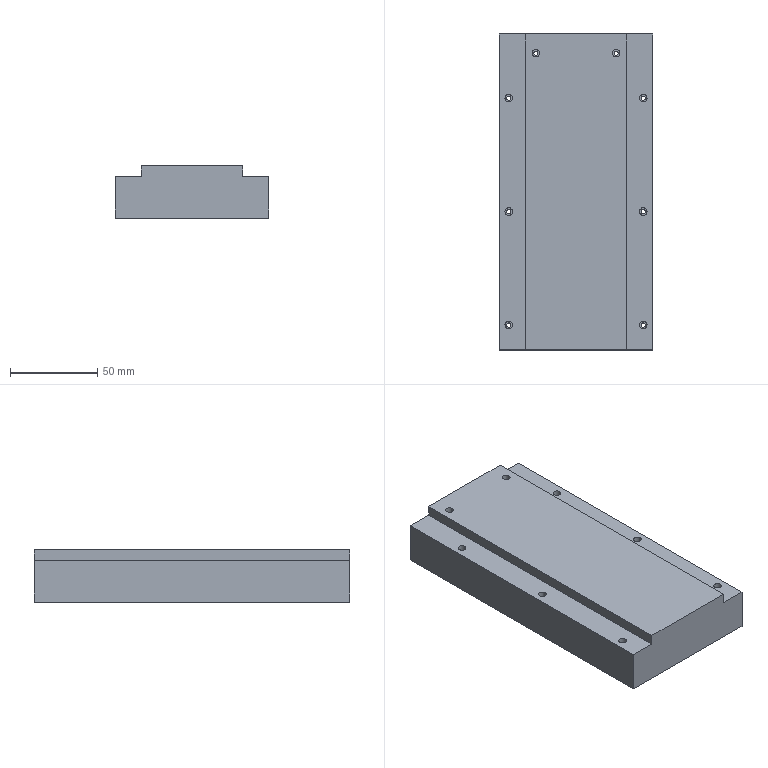NC program | NX | posted with a generic post | part box 88 x 181.05 x 30 mm
Whole program:
N10 G17 G21 G94 G90
(PLANAR_MILL , TOOL : D63_FACE_MILL)
N12 T01 M6
N14 G53
N16 G17 G0 G90 X-0.5 Y-125.025 B0. C0. S4500 M3
N18 G43 Z30. H1
N20 Z2.
N22 G94 G1 Z0. F1000.
N24 Y-90.525
N26 Y90.525
N28 Y125.025
N30 Z2.
N32 G0 Z30.
N34 M5
(DYNAMIC_ROUGH , TOOL : D16-48-D16-100-3T-ROUGH)
N36 T02 M6
N38 G53
N40 G17 G0 G90 X-57.579 Y-90.633 B0. C0. S5500 M3
N42 G43 Z30. H2
N44 Z-26.5
N46 G94 G1 X-57.554 Y-90.632 Z-26.656 F3000.
N48 X-57.529 Y-90.631 Z-26.718
N50 X-57.504 Y-90.63 Z-26.763
N52 X-57.479 Y-90.629 Z-26.8
N54 X-57.455 Y-90.627 Z-26.831
N56 X-57.43 Y-90.626 Z-26.857
N58 X-57.405 Y-90.625 Z-26.88
N60 X-57.38 Y-90.624 Z-26.9
N62 X-57.355 Y-90.623 Z-26.918
N64 X-57.33 Y-90.621 Z-26.933
N66 X-57.305 Y-90.62 Z-26.947
N68 X-57.28 Y-90.619 Z-26.958
N70 X-57.255 Y-90.618 Z-26.968
N72 X-57.23 Y-90.617 Z-26.977
N74 X-57.205 Y-90.616 Z-26.984
N76 X-57.18 Y-90.614 Z-26.99
N78 X-57.155 Y-90.613 Z-26.994
N80 X-57.13 Y-90.612 Z-26.997
N82 X-57.105 Y-90.611 Z-26.999
N84 X-57.08 Y-90.61 Z-27.
N86 X-54.472 Y-90.487
N88 G3 X-53.075 Y-89.537 R1.616
N90 X-52.43 Y-86.733 R10.15
N92 X-52.2 Y-83.934 R67.936
N94 G1 Y90.526
N96 G2 X-51.798 Y93.06 R9.591
N98 X-50.633 Y95.346 R9.588
N100 X-48.819 Y97.16 R9.588
N102 X-46.533 Y98.324 R9.588
N104 X-43.999 Y98.725 R9.593
N106 X-32.454 Y98.986 R196.191
N108 G1 X-20.754 Y98.999
N110 X41.21 Y99.
N112 G2 X43.288 Y98.73 R10.046
N114 X45.284 Y98.624 R17.692
N116 X47.724 Y97.831 R9.588
N118 X49.799 Y96.322 R9.588
N120 X51.307 Y94.247 R9.588
N122 X52.099 Y91.807 R9.588
N124 G1 X52.2 Y90.524
N126 Y-90.526
N128 G2 X51.798 Y-93.06 R9.591
N130 X50.633 Y-95.346 R9.588
N132 X48.819 Y-97.16 R9.588
N134 X46.533 Y-98.324 R9.588
N136 X43.999 Y-98.725 R9.593
N138 X32.154 Y-98.979 R208.552
N140 G1 X20.904 Y-98.992
N142 X-41.311 Y-98.998
N144 G2 X-43.313 Y-98.729 R10.858
N146 X-45.284 Y-98.624 R17.127
N148 X-47.724 Y-97.831 R9.588
N150 X-49.799 Y-96.322 R9.588
N152 X-51.307 Y-94.247 R9.588
N154 X-52.099 Y-91.807 R9.588
N156 G1 X-52.2 Y-90.524
N158 Y-83.924
N160 Y-90.524
N162 G3 X-51.799 Y-93.058 R9.591
N164 X-50.635 Y-95.344 R9.588
N166 X-48.821 Y-97.158 R9.588
N168 X-46.535 Y-98.323 R9.588
N170 X-44.001 Y-98.725 R9.59
N172 G1 X43.999
N174 G2 X45.055 Y-99.123 R1.603
N176 G1 X45.843 Y-99.815
N178 X48.221 Y-101.904 Z-26.9
N180 G3 X48.879 Y-102.348 R2.082 F15000.
N182 X50.166 Y-102.285 R1.602
N184 G1 X50.755 Y-101.993
N186 X51.337 Y-101.688
N188 G3 X52.586 Y-100.656 R5.048
N190 G1 X55.189 Y-97.678
N192 G3 X56.28 Y-95.623 R5.286
N194 X56.568 Y-94.077 R8.158
N196 G1 X56.754 Y-91.914
N198 X56.904 Y-89.749
N200 G3 X57.01 Y-86.198 R78.066
N202 G1 X58.009 Y83.924
N204 G3 X56.659 Y93.575 R33.76
N206 G1 X55.557 Y97.353
N208 G3 X54.581 Y99.002 R3.866
N210 X53.031 Y100.206 R7.93
N212 G1 X49.529 Y102.285
N214 G3 X47.677 Y102.129 R1.6
N216 G1 X45.351 Y99.983 Z-27. F3000.
N218 X44.84 Y99.506
N220 X44.317 Y99.041
N222 G2 X43.363 Y98.725 R1.605
N224 G1 X-43.999
N226 G2 X-45.511 Y99.769 R1.616
N228 G1 X-46.507 Y102.398
N230 X-46.516 Y102.422 Z-26.999
N232 X-46.525 Y102.445 Z-26.997
N234 X-46.533 Y102.468 Z-26.994
N236 X-46.542 Y102.492 Z-26.99
N238 X-46.551 Y102.515 Z-26.984
N240 X-46.56 Y102.539 Z-26.977
N242 X-46.569 Y102.562 Z-26.968
N244 X-46.578 Y102.585 Z-26.958
N246 X-46.587 Y102.609 Z-26.947
N248 X-46.595 Y102.632 Z-26.933
N250 X-46.604 Y102.655 Z-26.918
N252 X-46.613 Y102.679 Z-26.9
N254 X-46.622 Y102.702 Z-26.88
N256 X-46.631 Y102.726 Z-26.857
N258 X-46.64 Y102.749 Z-26.831
N260 X-46.649 Y102.772 Z-26.8
N262 X-46.657 Y102.796 Z-26.763
N264 X-46.666 Y102.819 Z-26.718
N266 X-46.675 Y102.842 Z-26.656
N268 X-46.684 Y102.866 Z-26.5
N270 G0 Z30.
N272 X-27.662 Y-103.175
N274 Z-5.4
N276 G1 X-27.665 Y-103.151 Z-5.556
N278 X-27.669 Y-103.126 Z-5.618
N280 X-27.672 Y-103.101 Z-5.663
N282 X-27.675 Y-103.076 Z-5.7
N284 X-27.679 Y-103.052 Z-5.731
N286 X-27.682 Y-103.027 Z-5.757
N288 X-27.686 Y-103.002 Z-5.78
N290 X-27.689 Y-102.977 Z-5.8
N292 X-27.692 Y-102.953 Z-5.818
N294 X-27.696 Y-102.928 Z-5.833
N296 X-27.699 Y-102.903 Z-5.847
N298 X-27.702 Y-102.878 Z-5.858
N300 X-27.706 Y-102.853 Z-5.868
N302 X-27.709 Y-102.829 Z-5.877
N304 X-27.713 Y-102.804 Z-5.884
N306 X-27.716 Y-102.779 Z-5.89
N308 X-27.719 Y-102.754 Z-5.894
N310 X-27.723 Y-102.73 Z-5.897
N312 X-27.726 Y-102.705 Z-5.899
N314 X-27.73 Y-102.68 Z-5.9
N316 X-28.086 Y-100.075
N318 G3 X-29.541 Y-98.685 R1.616
N320 G2 X-31.248 Y-98.389 R6.552
N322 G3 X-36.939 Y-97.859 R36.404
N324 G2 X-41.14 Y-97.737 R191.406
N326 X-46.63 Y-94.925 R8.88
N328 X-49.802 Y-89.208 R13.973
N330 X-50.922 Y-82.262 R31.9
N332 X-51.187 Y-71.017 R186.99
N334 G1 X-51.199 Y-61.042
N336 X-51.198 Y86.901
N338 G2 X-48.907 Y92.541 R8.533
N340 X-43.44 Y96.04 R13.087
N342 X-36.686 Y97.363 R27.458
N344 G1 X-33.393 Y97.572
N346 G3 X-32.896 Y97.734 R4.726
N348 X-32.094 Y98.834 R1.601
N350 G1 X-32.001 Y99.319
N352 X-31.402 Y102.427 Z-5.8
N354 X-31.332 Y102.782 F15000.
N356 X-31.277 Y103.139
N358 G3 X-32.896 Y104.854 R1.6
N360 X-33.667 Y104.739 R1.952
N362 X-33.623 Y101.747 R1.6
N364 X-32.812 Y101.666 Z-5.826 R1.799 F3000.
N366 G1 X-30.476 Y101.827 Z-5.9
N368 X-30.04 Y101.859
N370 X-29.604 Y101.876
N372 G2 X-29.541 Y98.685 R1.6
N374 G3 X-33.041 Y97.642 R7.836
N376 G2 X-35.701 Y97.035 R14.011
N378 G3 X-41.183 Y95.918 R44.607
N380 X-45.299 Y93.969 R12.692
N382 X-49.136 Y88.494 R11.803
N384 X-50.345 Y82.178 R23.998
N386 X-50.588 Y73.108 R134.382
N388 G1 X-50.599 Y64.183
N390 X-50.597 Y-64.942
N392 G3 X-50.43 Y-79.565 R388.114
N394 X-49.633 Y-86.636 R41.552
N396 X-47.833 Y-91.304 R14.579
N398 X-42.835 Y-95.395 R11.325
N400 X-37.277 Y-96.902 R22.176
N402 G2 X-33.43 Y-97.474 R557.51
N404 X-32.788 Y-97.798 R2.588
N406 G1 X-31.613 Y-98.297
N408 X-31.177 Y-98.407
N410 G2 X-33.401 Y-97.415 R7.129
N412 G3 X-36.273 Y-96.393 R15.382
N414 G2 X-40.738 Y-94.86 R28.115
N416 X-46.549 Y-89.135 R13.103
N418 X-48.77 Y-82.231 R22.213
N420 X-49.486 Y-73.341 R65.312
N422 X-49.598 Y-55.492 R785.745
N424 G1 X-49.597 Y67.108
N426 G2 X-49.452 Y79.106 R295.937
N428 X-48.643 Y85.266 R29.808
N430 X-43.491 Y92.428 R12.3
N432 X-37.725 Y95.096 R22.188
N434 G3 X-35.367 Y95.873 R98.773
N436 X-34.886 Y96.226 R2.627
N438 X-34.641 Y97.883 R1.6
N440 X-35.595 Y98.768 Z-5.858 R1.617
N442 G1 X-37.321 Y99.358 Z-5.8
N444 X-37.758 Y99.504 F15000.
N446 X-38.189 Y99.666
N448 G2 X-38.446 Y102.392 R1.6
N450 G1 X-38.155 Y102.61
N452 X-37.856 Y102.816
N454 G2 X-36.107 Y102.716 R1.6
N456 G1 X-34.381 Y101.44
N458 X-32.801 Y100.265 Z-5.862 F3000.
N460 G2 X-32.237 Y99.244 Z-5.9 R1.6
N462 X-32.976 Y97.68 R1.6
N464 G3 X-35.029 Y96.06 R7.847
N466 G2 X-36.762 Y95.084 R7.614
N468 G3 X-41.137 Y92.939 R42.882
N470 X-47.329 Y85.319 R14.067
N472 X-48.679 Y78.496 R26.941
N474 X-48.983 Y68.753 R129.201
N476 G1 X-48.998 Y59.078
N478 X-48.996 Y-59.172
N480 G3 X-48.83 Y-74.32 R437.01
N482 X-48.002 Y-82.37 R51.912
N484 X-45.631 Y-88.734 R19.104
N486 X-40.141 Y-93.77 R14.478
N488 X-35.55 Y-95.849 R48.344
N490 G2 X-34.858 Y-96.259 R2.394
N492 X-34.522 Y-97.637 R1.601
N494 X-34.98 Y-98.456 Z-5.87 R1.755
N496 G1 X-36.432 Y-100.128 Z-5.8
N498 X-38.327 Y-102.309 F15000.
N500 G3 X-36.849 Y-104.957 R1.604
N502 X-35.78 Y-104.232 R1.602
N504 G1 X-34.105 Y-101.558
N506 X-32.85 Y-99.544 Z-5.875 F3000.
N508 G3 X-32.648 Y-98.788 Z-5.9 R1.606
N510 X-33.401 Y-97.415 R1.601
N512 G2 X-35.029 Y-96.057 R7.102
N514 G3 X-37.102 Y-94.559 R13.304
N516 G2 X-41.245 Y-91.517 R25.827
N518 X-46.005 Y-83.797 R18.407
N520 X-47.566 Y-75.486 R36.355
N522 X-47.964 Y-64.396 R149.197
N524 G1 X-47.997 Y-49.846
N526 X-47.996 Y62.029
N528 G2 X-47.833 Y74.927 R309.518
N530 X-46.958 Y81.836 R36.18
N532 X-41.207 Y90.707 R15.688
N534 X-37.224 Y93.434 R49.413
N536 G3 X-36.32 Y94.219 R2.677
N538 X-36.485 Y95.731 R1.601
N540 X-37.618 Y96.419 Z-5.857 R1.679
N542 G1 X-39.379 Y96.791 Z-5.8
N544 X-39.912 Y96.9 F15000.
N546 X-40.441 Y97.027
N548 G2 X-41.355 Y99.254 R1.6
N550 G1 X-41.208 Y99.553
N552 X-41.048 Y99.845
N554 G2 X-38.979 Y100.384 R1.6
N556 G1 X-37.225 Y99.478
N558 X-35.394 Y98.527 Z-5.865 F3000.
N560 G2 X-34.7 Y97.701 Z-5.9 R1.601
N562 X-34.979 Y96.116 R1.601
N564 G1 X-35.657 Y95.312
N566 X-36.427 Y94.024
N568 G2 X-38.244 Y92.338 R11.446
N570 G3 X-42.213 Y88.719 R30.381
N572 X-46.224 Y80.707 R18.633
N574 X-47.202 Y73.131 R40.97
N576 X-47.393 Y61.059 R266.297
N578 G1 X-47.397 Y55.509
N580 X-47.395 Y-54.491
N582 G3 X-47.224 Y-70.539 R479.067
N584 X-46.319 Y-79.56 R59.081
N586 X-43.601 Y-86.988 R22.788
N588 X-38.701 Y-92.39 R20.469
N590 G2 X-36.307 Y-94.305 R71.67
N592 X-35.659 Y-95.311 R6.411
N594 G1 X-34.981 Y-96.113
N596 G2 X-36.154 Y-94.495 R7.587
N598 G3 X-38. Y-92.16 R13.26
N600 G2 X-41.934 Y-87.122 R30.771
N602 X-45.226 Y-78.145 R27.23
N604 X-46.199 Y-68.528 R64.957
N606 X-46.392 Y-53.68 R418.722
N608 G1 X-46.396 Y-47.23
N610 X-46.395 Y58.12
N612 G2 X-46.224 Y71.543 R328.441
N614 X-45.287 Y79.2 R41.789
N616 X-40.223 Y88.601 R20.398
N618 G3 X-37.288 Y91.723 R211.462
N620 X-36.977 Y92.317 R2.167
N622 G1 X-36.805 Y93.04
N624 X-36.32 Y94.221
N626 X-36.805 Y93.04
N628 G2 X-37.133 Y91.859 R5.847
N630 X-38.688 Y89.653 R14.553
N632 G3 X-42.088 Y84.891 R35.69
N634 X-45.011 Y76.194 R25.459
N636 X-45.709 Y67.003 R68.975
N638 X-45.796 Y52.153 R780.496
N640 G1 X-45.794 Y-50.872
N642 G3 X-45.618 Y-67.445 R507.889
N644 X-44.68 Y-77.216 R67.586
N646 X-41.201 Y-86.677 R27.532
N648 X-37.798 Y-91.331 R44.339
N650 G2 X-36.937 Y-92.557 R6.424
N652 G3 X-36.321 Y-94.219 R10.442
N654 G1 X-36.805 Y-93.038
N656 G3 X-37.803 Y-90.538 R7.763
N658 G2 X-40.562 Y-85.586 R97.842
N660 X-43.9 Y-74.327 R36.607
N662 X-44.68 Y-63.11 R97.377
N664 X-44.795 Y-42.861 R960.397
N666 G1 X-44.794 Y54.689
N668 G2 X-44.614 Y68.712 R346.85
N670 X-43.615 Y77.116 R47.758
N672 X-39.681 Y86.157 R27.035
N674 G3 X-37.365 Y89.78 R62.753
N676 X-37.2 Y90.526 R1.886
N678 G1 X-37.1 Y91.799
N680 X-36.996 Y92.236
N682 X-37.1 Y91.799
N684 G3 X-37.202 Y90.205 R30.629
N686 G2 X-38.003 Y88.147 R7.219
N688 G3 X-40.578 Y83.342 R148.541
N690 X-43.578 Y72.699 R33.082
N692 X-44.137 Y62.67 R96.58
N694 X-44.195 Y49.02 R824.817
N696 G1 X-44.193 Y-47.555
N698 G3 X-43.996 Y-65.253 R514.765
N700 X-42.956 Y-75.842 R73.395
N702 X-38.768 Y-87.44 R38.406
N704 G2 X-37.249 Y-90.463 R40.428
N706 X-37.101 Y-91.796 R7.37
N708 G1 X-36.962 Y-92.38
N710 G2 X-37.182 Y-90.755 R6.826
N712 G3 X-37.785 Y-88.183 R8.487
N714 G2 X-40. Y-82.353 R344.373
N716 X-42.626 Y-69.522 R52.699
N718 X-43.15 Y-56.035 R172.474
N720 G1 X-43.193 Y-42.985
N722 X-43.194 Y49.015
N724 G2 X-43.042 Y65.363 R503.011
N726 X-42.06 Y74.902 R59.741
N728 X-38.84 Y84.089 R37.509
N730 G3 X-37.263 Y87.577 R44.436
N732 G1 X-37.2 Y87.946
N734 Y90.346
N736 Y87.721
N738 G2 X-38.01 Y84.934 R11.897
N740 G3 X-40.253 Y78.95 R94.427
N742 X-42.228 Y67.976 R47.273
N744 X-42.58 Y55.233 R191.566
N746 G1 X-42.594 Y45.633
N748 X-42.592 Y-44.492
N750 G3 X-42.393 Y-62.94 R557.266
N752 X-41.306 Y-74.504 R84.598
N754 X-38.407 Y-84.74 R56.515
N756 G2 X-37.213 Y-88.338 R32.946
N758 G1 X-37.2 Y-90.513
N760 G3 X-37.227 Y-87.289 R48.809
N762 X-38.108 Y-83.238 R27.601
N764 G2 X-40.368 Y-73.316 R85.738
N766 X-41.424 Y-60.392 R104.045
N768 X-41.591 Y-42.244 R677.387
N770 G1 X-41.593 Y46.006
N772 G2 X-41.442 Y62.955 R552.269
N774 X-40.382 Y73.616 R68.567
N776 X-38.079 Y81.685 R54.328
N778 G3 X-37.217 Y84.299 R32.425
N780 X-37.2 Y87.748 R75.884
N782 G1 X-37.216 Y83.983
N784 G2 X-38.078 Y80.196 R25.33
N786 G3 X-40.743 Y64.073 R65.145
N788 X-40.988 Y49.527 R317.354
N790 G1 X-40.992 Y43.302
N792 X-40.991 Y-41.723
N794 G3 X-40.785 Y-61.071 R595.252
N796 X-39.534 Y-74.276 R96.031
N798 X-37.638 Y-82.619 R110.394
N800 G2 X-37.2 Y-84.591 R26.785
N802 G1 Y-87.666
N804 G3 X-37.221 Y-82.574 R148.285
N806 X-37.777 Y-78.578 R47.276
N808 G2 X-39.819 Y-58.523 R122.634
N810 X-39.99 Y-38.574 R784.404
N812 G1 X-39.992 Y43.751
N814 G2 X-39.821 Y61.299 R541.407
N816 X-38.553 Y73.521 R77.38
N818 X-37.213 Y79.398 R165.87
N820 G1 X-37.2 Y84.273
N822 X-37.213 Y78.685
N824 G2 X-37.956 Y73.588 R61.471
N826 G3 X-39.272 Y58.509 R103.852
N828 X-39.391 Y40.96 R809.745
N830 G1 Y-74.951
N832 G2 X-39.518 Y-75.575 R1.631
N834 G1 X-39.922 Y-76.529
N836 X-41.155 Y-79.444 Z-5.8
N838 X-41.338 Y-79.881 F15000.
N840 X-41.535 Y-80.311
N842 G2 X-42.951 Y-81.117 R1.601
N844 G1 X-44.078 Y-81.098
N846 G3 X-44.179 Y-84.296 R1.6
N848 G1 X-41.175 Y-84.434
N850 X-38.787 Y-84.539 Z-5.876 F3000.
N852 G3 X-38.044 Y-84.351 Z-5.9 R1.607
N854 X-37.2 Y-82.941 R1.601
N856 X-37.229 Y-78.107 R108.816
N858 X-38.004 Y-70.447 R255.912
N860 G2 X-38.337 Y-60.331 R110.883
N862 G1 X-38.341 Y-53.731
N864 X-38.34 Y70.926
N866 G3 X-38.436 Y71.471 R1.672
N868 G1 X-39.64 Y74.79
N870 X-39.97 Y75.705 Z-5.869
N872 X-40.309 Y76.617 Z-5.838
N874 G3 X-41.149 Y77.458 Z-5.8 R1.6
N876 X-43.375 Y75.961 R1.6 F15000.
N878 G1 X-43.372 Y75.577
N880 X-43.352 Y75.195
N882 G3 X-41.171 Y73.928 R1.6
N884 X-40.17 Y75.521 Z-5.864 R1.606 F3000.
N886 G1 X-40.249 Y76.671 Z-5.9
N888 X-40.396 Y78.839
N890 G2 X-37.2 Y78.948 R-1.6
N892 X-37.476 Y73.301 R40.731
N894 G3 X-37.727 Y64.157 R129.856
N896 G1 X-37.74 Y54.407
N898 X-37.736 Y-70.751
N900 G2 X-37.2 Y-73.643 R55.721
N902 G1 Y-78.668
N904 Y76.807
N906 G3 X-38.586 Y78.407 R1.616
N908 G1 X-41.156 Y78.777
N910 X-41.181 Y78.781 Z-5.899
N912 X-41.205 Y78.784 Z-5.897
N914 X-41.23 Y78.788 Z-5.894
N916 X-41.255 Y78.791 Z-5.89
N918 X-41.279 Y78.795 Z-5.884
N920 X-41.304 Y78.798 Z-5.877
N922 X-41.329 Y78.802 Z-5.868
N924 X-41.354 Y78.806 Z-5.858
N926 X-41.378 Y78.809 Z-5.847
N928 X-41.403 Y78.813 Z-5.833
N930 X-41.428 Y78.816 Z-5.818
N932 X-41.453 Y78.82 Z-5.8
N934 X-41.477 Y78.823 Z-5.78
N936 X-41.502 Y78.827 Z-5.757
N938 X-41.527 Y78.831 Z-5.731
N940 X-41.552 Y78.834 Z-5.7
N942 X-41.576 Y78.838 Z-5.663
N944 X-41.601 Y78.841 Z-5.618
N946 X-41.626 Y78.845 Z-5.556
N948 X-41.651 Y78.848 Z-5.4
N950 G0 Z30.
N952 X27.662 Y103.175
N954 Z-5.4
N956 G1 X27.665 Y103.151 Z-5.556
N958 X27.669 Y103.126 Z-5.618
N960 X27.672 Y103.101 Z-5.663
N962 X27.675 Y103.076 Z-5.7
N964 X27.679 Y103.052 Z-5.731
N966 X27.682 Y103.027 Z-5.757
N968 X27.686 Y103.002 Z-5.78
N970 X27.689 Y102.977 Z-5.8
N972 X27.692 Y102.953 Z-5.818
N974 X27.696 Y102.928 Z-5.833
N976 X27.699 Y102.903 Z-5.847
N978 X27.702 Y102.878 Z-5.858
N980 X27.706 Y102.853 Z-5.868
N982 X27.709 Y102.829 Z-5.877
N984 X27.713 Y102.804 Z-5.884
N986 X27.716 Y102.779 Z-5.89
N988 X27.719 Y102.754 Z-5.894
N990 X27.723 Y102.73 Z-5.897
N992 X27.726 Y102.705 Z-5.899
N994 X27.73 Y102.68 Z-5.9
N996 X28.086 Y100.075
N998 G3 X29.541 Y98.685 R1.616
N1000 G2 X31.248 Y98.389 R6.552
N1002 G3 X36.543 Y97.876 R34.52
N1004 G2 X41.088 Y97.742 R627.78
N1006 X46.582 Y94.936 R8.89
N1008 X49.741 Y89.336 R13.941
N1010 X50.901 Y82.473 R30.771
N1012 X51.183 Y71.828 R166.117
N1014 G1 X51.199 Y61.028
N1016 Y-86.851
N1018 G2 X48.762 Y-92.735 R8.576
N1020 X43.264 Y-96.124 R13.244
N1022 X36.572 Y-97.379 R28.234
N1024 G1 X33.355 Y-97.582
N1026 G3 X32.86 Y-97.752 R4.815
N1028 X32.155 Y-98.736 R1.602
N1030 G1 X32.002 Y-99.379
N1032 X31.268 Y-102.457 Z-5.8
N1034 X31.191 Y-102.774 F15000.
N1036 X31.127 Y-103.094
N1038 G3 X32.86 Y-104.873 R1.6
N1040 X33.479 Y-104.77 R2.34
N1042 X33.563 Y-101.776 R1.6
N1044 X32.695 Y-101.672 Z-5.828 R1.773 F3000.
N1046 G1 X30.42 Y-101.831 Z-5.9
N1048 X30.013 Y-101.862
N1050 X29.605 Y-101.876
N1052 G2 X29.541 Y-98.685 R1.6
N1054 G3 X33.041 Y-97.642 R7.841
N1056 G2 X35.714 Y-97.039 R14.327
N1058 G3 X41.196 Y-95.932 R45.055
N1060 X45.428 Y-93.896 R12.469
N1062 X49.132 Y-88.537 R11.814
N1064 X50.344 Y-82.222 R23.955
N1066 X50.587 Y-73.228 R132.894
N1068 G1 X50.599 Y-64.453
N1070 X50.597 Y64.897
N1072 G3 X50.447 Y79.071 R418.723
N1074 X49.675 Y86.371 R44.128
N1076 X47.797 Y91.325 R15.044
N1078 X42.739 Y95.43 R11.289
N1080 X37.176 Y96.918 R22.397
N1082 G2 X33.419 Y97.477 R241.725
N1084 X32.788 Y97.798 R2.67
N1086 G1 X31.613 Y98.297
N1088 X31.177 Y98.407
N1090 G2 X33.391 Y97.421 R7.119
N1092 G3 X36.355 Y96.369 R15.586
N1094 G2 X40.792 Y94.826 R26.912
N1096 X46.558 Y89.092 R13.158
N1098 X48.772 Y82.191 R22.279
N1100 X49.48 Y73.527 R64.425
N1102 X49.598 Y57.403 R667.953
N1104 G1 Y-64.747
N1106 G2 X49.475 Y-78.621 R416.586
N1108 X48.752 Y-84.87 R33.205
N1110 X43.453 Y-92.472 R12.305
N1112 X37.733 Y-95.102 R22.213
N1114 G3 X35.371 Y-95.875 R182.58
N1116 X34.887 Y-96.224 R2.691
N1118 X34.641 Y-97.883 R1.6
N1120 X35.595 Y-98.768 Z-5.858 R1.617
N1122 G1 X37.322 Y-99.357 Z-5.8
N1124 X37.758 Y-99.504 F15000.
N1126 X38.188 Y-99.665
N1128 G2 X38.447 Y-102.391 R1.6
N1130 G1 X38.156 Y-102.609
N1132 X37.856 Y-102.816
N1134 G2 X36.106 Y-102.716 R1.6
N1136 G1 X34.381 Y-101.44
N1138 X32.801 Y-100.265 Z-5.862 F3000.
N1140 G2 X32.237 Y-99.243 Z-5.9 R1.6
N1142 X32.976 Y-97.68 R1.6
N1144 G3 X35.029 Y-96.06 R7.891
N1146 G2 X36.95 Y-95.004 R8.663
N1148 G3 X41.323 Y-92.84 R37.076
N1150 X47.332 Y-85.335 R14.038
N1152 X48.693 Y-78.362 R27.229
N1154 X48.983 Y-68.844 R131.936
N1156 G1 X48.998 Y-59.169
N1158 X48.996 Y58.856
N1160 G3 X48.829 Y74.304 R444.778
N1162 X47.969 Y82.5 R51.129
N1164 X45.548 Y88.847 R18.885
N1166 X39.975 Y93.855 R14.629
N1168 X35.508 Y95.866 R51.692
N1170 G2 X34.879 Y96.238 R2.518
N1172 X34.497 Y97.714 R1.601
N1174 X35.196 Y98.69 Z-5.861 R1.695
N1176 G1 X36.734 Y99.867 Z-5.8
N1178 X37.863 Y100.73 F15000.
N1180 G3 X38.426 Y102.456 R1.603
N1182 X35.632 Y103.057 R1.6
N1184 G1 X34.341 Y101.456
N1186 X32.943 Y99.714 Z-5.871 F3000.
N1188 G3 X32.64 Y98.849 Z-5.9 R1.603
N1190 X33.391 Y97.421 R1.601
N1192 G2 X35.029 Y96.057 R7.112
N1194 G3 X37.057 Y94.584 R12.939
N1196 G2 X41.164 Y91.585 R26.33
N1198 X45.966 Y83.895 R18.379
N1200 X47.548 Y75.664 R35.768
N1202 X47.963 Y64.424 R145.593
N1204 G1 X47.997 Y49.875
N1206 X47.996 Y-62.075
N1208 G2 X47.828 Y-75.048 R303.462
N1210 X46.915 Y-82.027 R35.159
N1212 X41.153 Y-90.763 R15.679
N1214 X37.165 Y-93.482 R52.04
N1216 G3 X36.304 Y-94.247 R2.491
N1218 G2 X34.931 Y-96.172 R9.009
N1220 G3 X36.304 Y-94.247 R9.039
N1222 G2 X37.117 Y-93.3 R3.297
N1224 G1 X40.343 Y-90.602
N1226 G3 X46.163 Y-80.972 R18.329
N1228 X47.205 Y-73.103 R40.233
N1230 X47.393 Y-61.106 R268.747
N1232 G1 X47.397 Y-55.556
N1234 X47.395 Y54.519
N1236 G3 X47.221 Y70.567 R473.769
N1238 X46.31 Y79.587 R58.808
N1240 X43.532 Y87.087 R22.654
N1242 X38.699 Y92.387 R20.534
N1244 G2 X36.336 Y94.272 R349.742
N1246 X35.659 Y95.311 R7.101
N1248 G1 X34.981 Y96.113
N1250 G2 X36.148 Y94.504 R7.558
N1252 G3 X37.989 Y92.168 R13.256
N1254 G2 X42.002 Y86.996 R30.481
N1256 X45.223 Y78.14 R27.313
N1258 X46.199 Y68.523 R64.871
N1260 X46.391 Y53.75 R414.218
N1262 G1 X46.396 Y47.225
N1264 X46.395 Y-58.2
N1266 G2 X46.213 Y-71.773 R314.86
N1268 X45.22 Y-79.496 R40.261
N1270 X40.26 Y-88.57 R20.315
N1272 G3 X37.264 Y-91.758 R206.313
N1274 X36.978 Y-92.312 R2.424
N1276 G1 X36.805 Y-93.04
N1278 X36.32 Y-94.221
N1280 X36.805 Y-93.04
N1282 G2 X37.133 Y-91.863 R5.732
N1284 X38.693 Y-89.654 R14.741
N1286 G3 X42.116 Y-84.857 R35.229
N1288 X45.021 Y-76.153 R25.489
N1290 X45.712 Y-66.886 R69.977
N1292 X45.796 Y-52.111 R799.078
N1294 G1 X45.794 Y50.839
N1296 G3 X45.618 Y67.412 R508.303
N1298 X44.723 Y76.962 R68.853
N1300 X41.451 Y86.251 R27.994
N1302 X37.889 Y91.212 R40.398
N1304 G2 X36.962 Y92.497 R8.541
N1306 G3 X36.321 Y94.219 R12.516
N1308 G1 X36.805 Y93.038
N1310 G3 X37.862 Y90.43 R8.113
N1312 G2 X40.68 Y85.336 R83.784
N1314 X43.907 Y74.272 R36.784
N1316 X44.681 Y63.055 R97.954
N1318 X44.795 Y42.731 R965.467
N1320 G1 X44.794 Y-54.669
N1322 G2 X44.619 Y-68.617 R354.967
N1324 X43.672 Y-76.878 R48.986
N1326 X39.697 Y-86.142 R26.952
N1328 G3 X37.373 Y-89.77 R65.981
N1330 X37.2 Y-90.526 R1.874
N1332 G1 X37.1 Y-91.799
N1334 X36.996 Y-92.237
N1336 X37.1 Y-91.799
N1338 G3 X37.202 Y-90.193 R32.486
N1340 G2 X38.015 Y-88.131 R7.559
N1342 G3 X40.597 Y-83.314 R138.376
N1344 X43.566 Y-72.815 R32.949
N1346 X44.136 Y-62.711 R95.406
N1348 X44.195 Y-48.386 R847.301
N1350 G1 X44.193 Y47.364
N1352 G3 X44.009 Y64.912 R539.736
N1354 X43.002 Y75.581 R75.896
N1356 X38.747 Y87.472 R38.588
N1358 G2 X37.233 Y90.513 R30.005
N1360 X37.101 Y91.796 R9.107
N1362 G1 X36.962 Y92.38
N1364 G2 X37.183 Y90.743 R6.891
N1366 G3 X37.776 Y88.201 R8.423
N1368 G2 X39.892 Y82.653 R627.127
N1370 X42.602 Y69.769 R52.175
N1372 X43.144 Y56.659 R163.853
N1374 X43.193 Y42.934 R886.056
N1376 G1 X43.194 Y-48.691
N1378 G2 X43.049 Y-65.19 R533.095
N1380 X42.112 Y-74.658 R61.228
N1382 X38.989 Y-83.786 R36.599
N1384 G3 X37.26 Y-87.594 R45.39
N1386 G1 X37.2 Y-87.963
N1388 Y-90.288
N1390 Y-87.738
N1392 G2 X38.021 Y-84.915 R11.769
N1394 G3 X40.334 Y-78.709 R88.089
N1396 X42.237 Y-67.872 R47.671
N1398 X42.579 Y-55.279 R194.072
N1400 G1 X42.594 Y-45.679
N1402 X42.592 Y44.446
N1404 G3 X42.397 Y62.819 R564.791
N1406 X41.299 Y74.533 R84.986
N1408 X38.625 Y84.134 R54.44
N1410 G2 X37.218 Y88.301 R43.745
N1412 X37.2 Y90.478 R53.698
N1414 G1 X37.214 Y87.417
N1416 G3 X38.012 Y83.588 R23.777
N1418 G2 X40.128 Y74.743 R97.896
N1420 X41.375 Y61.838 R93.104
N1422 X41.589 Y43.915 R528.791
N1424 G1 X41.593 Y37.315
N1426 X41.592 Y-48.385
N1428 G2 X41.397 Y-64.132 R403.887
N1430 X40.162 Y-74.697 R61.584
N1432 X37.878 Y-82.264 R61.028
N1434 G3 X37.209 Y-84.363 R16.695
N1436 G1 X37.2 Y-87.764
N1438 G2 X37.22 Y-83.923 R100.459
N1440 X38.026 Y-80.394 R25.08
N1442 G3 X40.291 Y-69.659 R65.632
N1444 X40.922 Y-58.506 R112.739
N1446 X40.993 Y-43.207 R858.341
N1448 G1 X40.991 Y41.743
N1450 G3 X40.786 Y61.016 R595.386
N1452 X39.555 Y74.149 R96.628
N1454 X37.635 Y82.62 R109.055
N1456 G2 X37.2 Y84.584 R23.554
N1458 G1 Y87.659
N1460 G3 X37.224 Y82.531 R132.32
N1462 X38.087 Y76.772 R68.277
N1464 G2 X39.813 Y58.721 R120.013
N1466 X39.99 Y39.223 R742.571
N1468 G1 X39.992 Y-43.702
N1470 G2 X39.818 Y-61.4 R542.426
N1472 X38.478 Y-73.914 R76.332
N1474 X37.207 Y-79.456 R268.848
N1476 G1 X37.2 Y-84.181
N1478 X37.21 Y-78.757
N1480 G2 X37.852 Y-74.229 R50.064
N1482 G3 X39.271 Y-58.558 R103.393
N1484 X39.391 Y-39.659 R867.629
N1486 G1 Y73.301
N1488 G2 X39.481 Y73.828 R1.684
N1490 G1 X40.096 Y75.592
N1492 X41.087 Y78.434 Z-5.805
N1494 X41.145 Y78.578 Z-5.8
N1496 G2 X42.952 Y79.467 R1.6 F15000.
N1498 G1 X43.252 Y79.399
N1500 X43.554 Y79.342
N1502 G3 X44.323 Y82.416 R1.6
N1504 G1 X41.175 Y83.695
N1506 X39.318 Y84.445 Z-5.863 F3000.
N1508 G3 X38.183 Y84.41 Z-5.9 R1.6
N1510 X37.2 Y82.934 R1.6
N1512 X37.226 Y78.182 R122.277
N1514 X37.972 Y70.77 R205.442
N1516 G2 X38.337 Y60.355 R105.883
N1518 G1 X38.341 Y53.455
N1520 Y-70.976
N1522 G3 X38.436 Y-71.521 R1.672
N1524 G1 X39.64 Y-74.841
N1526 X39.97 Y-75.756 Z-5.869
N1528 X40.309 Y-76.668 Z-5.838
N1530 G3 X41.149 Y-77.509 Z-5.8 R1.6
N1532 X43.376 Y-76.011 R1.6 F15000.
N1534 G1 X43.372 Y-75.631
N1536 X43.352 Y-75.253
N1538 G3 X41.171 Y-73.986 R1.6
N1540 X40.17 Y-75.58 Z-5.864 R1.606 F3000.
N1542 G1 X40.249 Y-76.73 Z-5.9
N1544 X40.396 Y-78.897
N1546 G2 X37.2 Y-79.006 R-1.6
N1548 X37.454 Y-73.573 R36.404
N1550 G3 X37.722 Y-65.18 R111.834
N1552 G1 X37.74 Y-54.38
N1554 X37.736 Y69.176
N1556 G2 X37.2 Y72.876 R223.56
N1558 G1 Y78.801
N1560 Y-76.824
N1562 G3 X38.586 Y-78.424 R1.616
N1564 G1 X41.156 Y-78.794
N1566 X41.181 Y-78.797 Z-5.899
N1568 X41.205 Y-78.801 Z-5.897
N1570 X41.23 Y-78.804 Z-5.894
N1572 X41.255 Y-78.808 Z-5.89
N1574 X41.279 Y-78.812 Z-5.884
N1576 X41.304 Y-78.815 Z-5.877
N1578 X41.329 Y-78.819 Z-5.868
N1580 X41.354 Y-78.822 Z-5.858
N1582 X41.378 Y-78.826 Z-5.847
N1584 X41.403 Y-78.829 Z-5.833
N1586 X41.428 Y-78.833 Z-5.818
N1588 X41.453 Y-78.836 Z-5.8
N1590 X41.477 Y-78.84 Z-5.78
N1592 X41.502 Y-78.844 Z-5.757
N1594 X41.527 Y-78.847 Z-5.731
N1596 X41.552 Y-78.851 Z-5.7
N1598 X41.576 Y-78.854 Z-5.663
N1600 X41.601 Y-78.858 Z-5.618
N1602 X41.626 Y-78.861 Z-5.556
N1604 X41.651 Y-78.865 Z-5.4
N1606 G0 Z30.
N1608 M5
(PLANAR_MILL_1 , TOOL : D16-48-D16-100-3T-FINISH)
N1610 T03 M6
N1612 G53
N1614 G17 G0 G90 X-43.4 Y-106.525 B0. C0. S4500 M3
N1616 G43 Z30. H3
N1618 Z-3.
N1620 G94 G1 Z-6. F1000.
N1622 Y-90.525
N1624 Y90.525
N1626 Y106.525
N1628 Z-3.
N1630 G0 Z30.
N1632 X-37. Y-106.525
N1634 Z-3.
N1636 G1 Z-6.
N1638 Y-90.525
N1640 Y90.525
N1642 Y106.525
N1644 Z-3.
N1646 G0 Z30.
N1648 X43.4
N1650 Z-3.
N1652 G1 Z-6.
N1654 Y90.525
N1656 Y-90.525
N1658 Y-106.525
N1660 Z-3.
N1662 G0 Z30.
N1664 X37. Y106.525
N1666 Z-3.
N1668 G1 Z-6.
N1670 Y90.525
N1672 Y-90.525
N1674 Y-106.525
N1676 Z-3.
N1678 G0 Z30.
(PLANAR_MILL_1_COPY , TOOL : D16-48-D16-100-3T-FINISH)
N1680 X-57.856 Y98.525
N1682 Z-24.
N1684 G1 Z-27.
N1686 X-43.997
N1688 X44.
N1690 G2 X52. Y90.525 R8.
N1692 G1 Y-90.525
N1694 G2 X44. Y-98.525 R8.
N1696 G1 X-44.
N1698 G2 X-52. Y-90.525 R8.
N1700 G1 Y90.522
N1702 Y104.381
N1704 Z-24.
N1706 G0 Z30.
N1708 M5
(DRILLING , TOOL : CHAMFER_D6-90DEG)
N1710 T04 M6
N1712 G53
N1714 G17 G0 G90 X23. Y79.525 B0. C0. S3000 M3
N1716 G43 Z30. H4
N1718 G94 G81 G99 Z-2.2 F200. R3.
N1720 X-23.
N1722 G80
N1724 G0 X-23. Y79.525 Z30.
(DRILLING_COPY , TOOL : CHAMFER_D6-90DEG)
N1726 X38.5 Y53.775
N1728 G81 G98 Z-8.2 F200. R-3.
N1730 Y-11.225
N1732 Y-76.225
N1734 X-38.5
N1736 Y-11.225
N1738 Y53.775
N1740 G80
N1742 G0 X-38.5 Y53.775 Z30.
(PLANAR_MILL_2 , TOOL : CHAMFER_D6-90DEG)
N1744 X31. Y95.108
N1746 Z1.
N1748 G1 Z-2. F1000.
N1750 Y90.524
N1752 Y-90.525
N1754 G2 X29. Y-92.525 R2.
N1756 G1 X-29.
N1758 G2 X-31. Y-90.525 R2.
N1760 G1 Y90.525
N1762 G2 X-29. Y92.525 R2.
N1764 G1 X28.999
N1766 X33.583
N1768 Z1.
N1770 G0 Z30.
N1772 M5
(DRILLING_1_COPY_1 , TOOL : DRILL_D4.2-54-83)
N1774 T05 M6
N1776 G53
N1778 G17 G0 G90 X23. Y79.525 B0. C0. S3000 M3
N1780 G43 Z30. H5
N1782 G94 G83 G99 Z-25.8 F200. Q3. R3.
N1784 X-23.
N1786 G80
N1788 G0 X-23. Y79.525 Z30.
(DRILLING_1_COPY_COPY , TOOL : DRILL_D4.2-54-83)
N1790 X38.5 Y53.775
N1792 G83 G98 Z-25.8 F200. Q3. R-3.
N1794 Y-11.225
N1796 Y-76.225
N1798 X-38.5
N1800 Y-11.225
N1802 Y53.775
N1804 G80
N1806 G0 X-38.5 Y53.775 Z30.
N1808 M5
(DRILLING_1 , TOOL : DRILL_D2.4-29-55)
N1810 T07 M6
N1812 G53
N1814 G17 G0 G90 X23. Y79.525 B0. C0. S3000 M3
N1816 G43 Z30. H7
N1818 G94 G81 G98 Z-33. F150. R-22.
N1820 X-23.
N1822 G80
N1824 G0 X-23. Y79.525 Z30.
(DRILLING_1_COPY , TOOL : DRILL_D2.4-29-55)
N1826 X-38.5 Y53.775
N1828 G81 Z-32.221 F150. R-22.
N1830 Y-11.225
N1832 Y-76.225
N1834 X38.5
N1836 Y-11.225
N1838 Y53.775
N1840 G80
N1842 G0 X38.5 Y53.775 Z30.
N1844 M5
(DRILLING_1_COPY_COPY_COPY , TOOL : D4.2)
N1846 T00 M6
N1848 G53
N1850 G17 G0 G90 X38.5 Y53.775 B0. C0. S1600 M3
N1852 G43 Z30. H1
N1854 G94 G81 G98 Z-25. F100. R-3.
N1856 Y-11.225
N1858 Y-76.225
N1860 X-38.5
N1862 Y-11.225
N1864 Y53.775
N1866 G80
N1868 G0 X-38.5 Y53.775 Z30.
(DRILLING_1_COPY_1_COPY , TOOL : D4.2)
N1870 X23. Y79.525
N1872 G81 G99 Z-25. F100. R3.
N1874 X-23.
N1876 G80
N1878 G0 X-23. Y79.525 Z30.
N1880 M5
N1882 M2